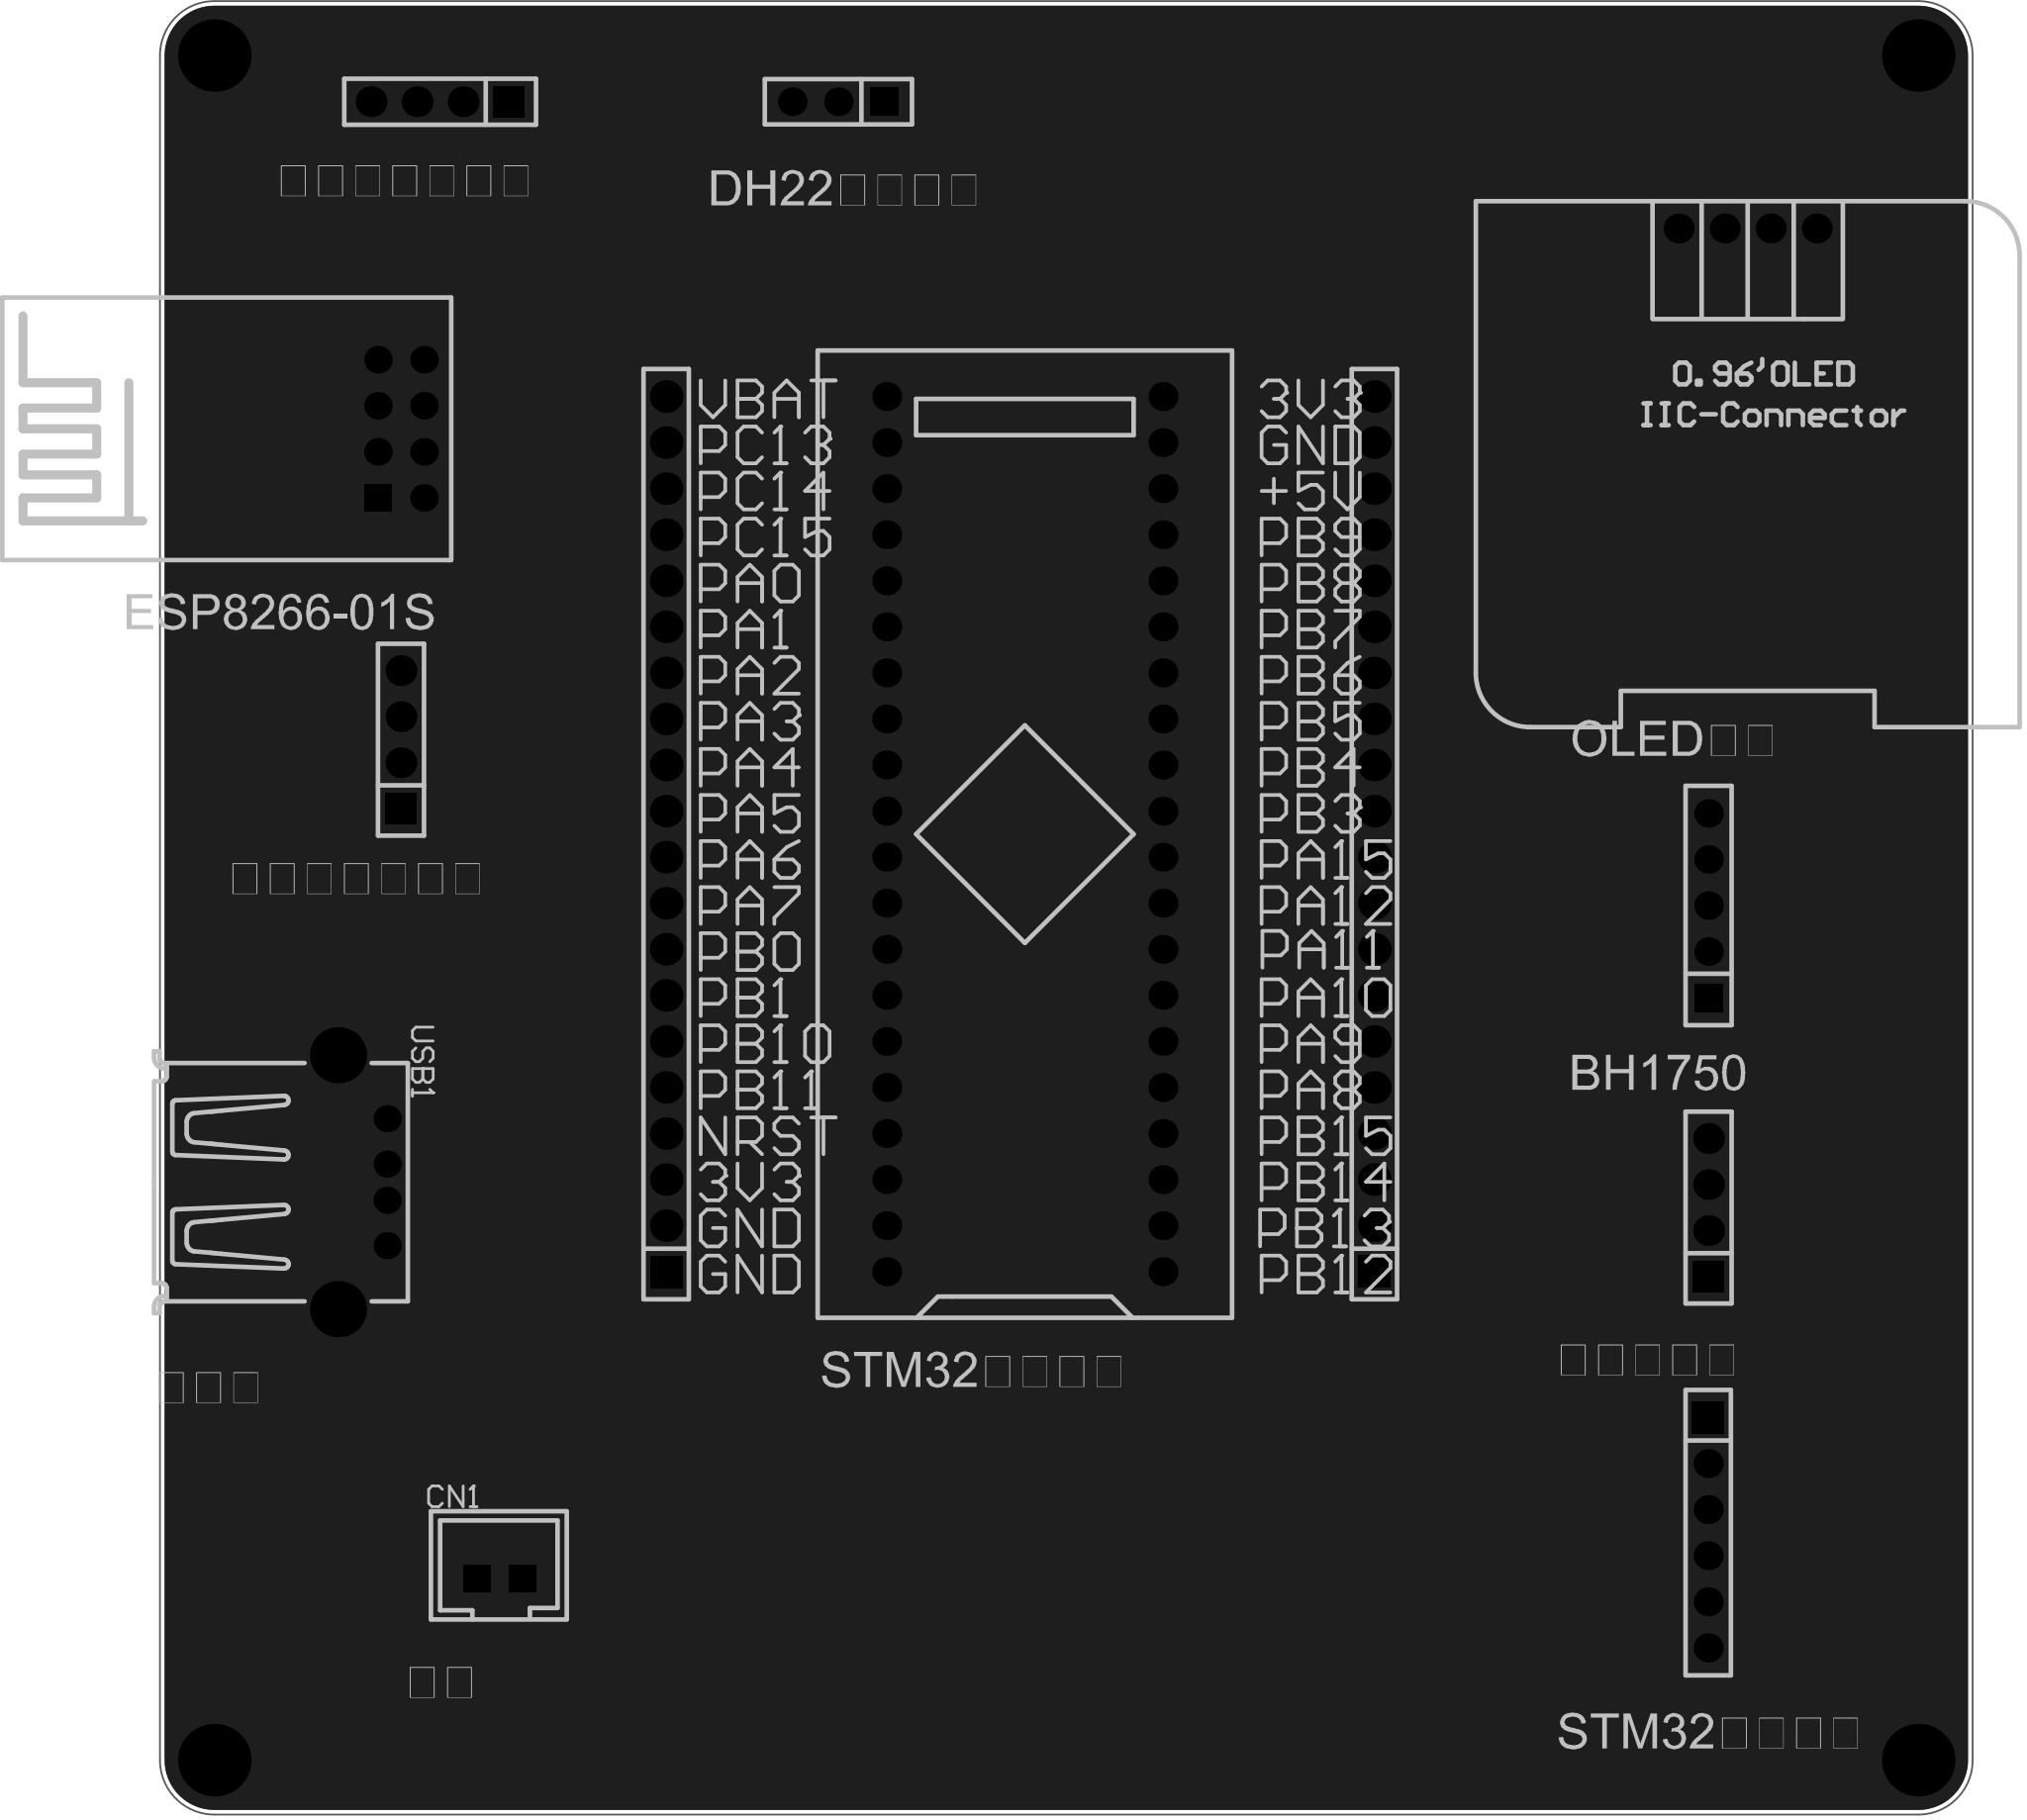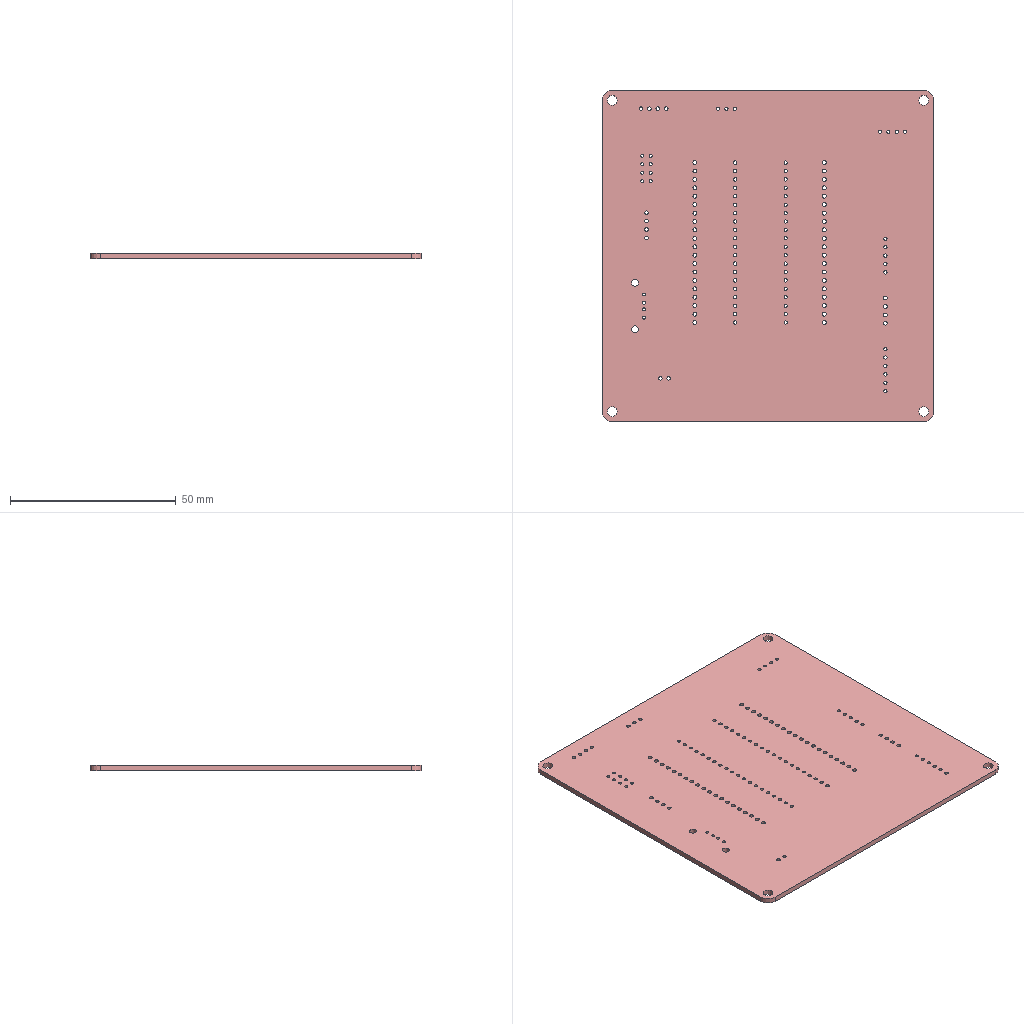Circuit board layout | Altium Designer | box 100 x 100 x 1.6 mm
Layer stack:
# Altium Designer layer stack of  (unit mm; dielectric type: 0 none, 1 core, 2 prepreg, 3 surface material)
index,name,kind,layer,copper_thickness_mm,dielectric_type,dielectric_thickness_mm,dielectric_material,dielectric_constant
0,Top Paste Mask Layer,other,,,,,,
1,Top Silkscreen Layer,other,,,,,,
2,Top Solder Mask Layer,dielectric,,,3,0.01,,3.3
3,Top Layer,copper,Top Layer,0.035,,,,
4,Dielectric1,dielectric,,,3,1.51,FR4,4.5
5,Bottom Layer,copper,Bottom Layer,0.035,,,,
6,Bottom Solder Mask Layer,dielectric,,,3,0.01,,3.3
7,Bottom Silkscreen Layer,other,,,,,,
8,Bottom Paste Mask Layer,other,,,,,,
# drill layer pairs: low layer,high layer
drill_pair,Top Layer,Bottom Layer
Part placement:
Designator,Comment,Layer,Footprint,Center-X(mm),Center-Y(mm),Rotation
U1,STM32F103C8T6-Card,TopLayer,CONN-TH_L53.3-W22.9_STM32F103C8T6-CARD,132.612,132.969,90
OLED1,,TopLayer,0.96OLED_4P,172.49,166.37,0
H28,,TopLayer,HDR-TH_4P-P2.54-V-F,98.195,138.176,90
H15,,TopLayer,HDR-TH_3P-P2.54-V-F,122.325,173.355,180
H1,,TopLayer,HDR-TH_20P-P2.54-V-F,151.895,132.969,90
H2,,TopLayer,HDR-TH_20P-P2.54-V-F,112.824,132.969,90
CN1,XH2.54-2PIN-直针,TopLayer,CONN-TH_XH2.54-2P,103.656,91.948,0
H26,,TopLayer,HDR-TH_4P-P2.54-V-F,100.354,173.355,180
H27,,TopLayer,HDR-TH_5P-P2.54-V-F,170.331,129.032,90
H29,,TopLayer,HDR-TH_4P-P2.54-V-F,170.331,112.376,90
H30,,TopLayer,HDR-TH_6P-P2.54-V-F,170.311,94.451,270
U2,ESP8266-01S,TopLayer,WIFIM-TH_ESP8266-01S,98.195,155.321,90
USB1,,TopLayer,USB__Type-A,96.078,113.776,270
Pad and via stacks:
# Altium Designer via and pad stacks of  (unit mm). Each distinct definition once, with the count of objects using it.
# via: kind,start_layer,end_layer,hole_mm,diameter_mm,mode(0 simple;1 top-mid-bottom;2 full stack),diameter_per_layer,count,example_net
# pad: kind,layer,hole_mm,hole_type(0 round;1 square;2 slot),plating,top_size,top_shape(1 round;2 rect;3 octagon;9 rounded rect),mid_size,bottom_size,mode,footprint,size_per_layer,count,example
pad,Multi-Layer,3,0,plated,4x4,1,4x4,4x4,0,,,4,1
pad,Multi-Layer,1,0,plated,1.6x1.6,1,1.6x1.6,1.6x1.6,0,CONN-TH_L53.3-W22.9_STM32F103C8T6-CARD,,40,U1.1
pad,Multi-Layer,1,0,plated,1.65x1.65,1,1.65x1.65,1.65x1.65,0,0.96OLED_4P,,4,OLED1.4
pad,Multi-Layer,1.1,0,plated,1.7x1.7,2,1.7x1.7,1.7x1.7,0,HDR-TH_4P-P2.54-V-F,,3,H28.1
pad,Multi-Layer,1.1,0,plated,1.7x1.7,1,1.7x1.7,1.7x1.7,0,HDR-TH_4P-P2.54-V-F,,9,H28.2
pad,Multi-Layer,1.02,0,plated,1.575x1.575,1,1.575x1.575,1.575x1.575,0,HDR-TH_3P-P2.54-V-F,,2,H15.3
pad,Multi-Layer,1.02,0,plated,1.575x1.575,2,1.575x1.575,1.575x1.575,0,HDR-TH_3P-P2.54-V-F,,1,H15.1
pad,Multi-Layer,1.2,0,plated,1.8x1.8,2,1.8x1.8,1.8x1.8,0,HDR-TH_20P-P2.54-V-F,,2,H1.1
pad,Multi-Layer,1.2,0,plated,1.8x1.8,1,1.8x1.8,1.8x1.8,0,HDR-TH_20P-P2.54-V-F,,38,H1.2
pad,Multi-Layer,1,2,plated,1.524x1.524,2,1.524x1.524,1.524x1.524,0,CONN-TH_XH2.54-2P,,2,CN1.1
pad,Multi-Layer,1.02,0,plated,1.575x1.575,1,1.575x1.575,1.575x1.575,0,HDR-TH_5P-P2.54-V-F,,4,H27.5
pad,Multi-Layer,1.02,0,plated,1.575x1.575,2,1.575x1.575,1.575x1.575,0,HDR-TH_5P-P2.54-V-F,,1,H27.1
pad,Multi-Layer,1.02,0,plated,1.6x1.6,1,1.6x1.6,1.6x1.6,0,HDR-TH_6P-P2.54-V-F,,5,H30.6
pad,Multi-Layer,1.02,0,plated,1.8x1.8,2,1.8x1.8,1.8x1.8,0,HDR-TH_6P-P2.54-V-F,,1,H30.1
pad,Multi-Layer,0.9144,0,plated,1.524x1.524,1,1.524x1.524,1.524x1.524,0,WIFIM-TH_ESP8266-01S,,7,U2.8
pad,Multi-Layer,0.9144,0,plated,1.524x1.524,2,1.524x1.524,1.524x1.524,0,WIFIM-TH_ESP8266-01S,,1,U2.1
pad,Multi-Layer,2.1,0,plated,3.1x3.1,1,3.1x3.1,3.1x3.1,0,USB_ Type-A,,2,USB1.SH2
pad,Multi-Layer,0.9,0,plated,1.5x1.5,1,1.5x1.5,1.5x1.5,0,USB_ Type-A,,4,USB1.1
Copper pours:
name,layer,net,type(0 solid;1 hatched;2 none)
Bottom Layer-GND,Bottom Layer,GND,0
Top Layer-GND,Top Layer,GND,0